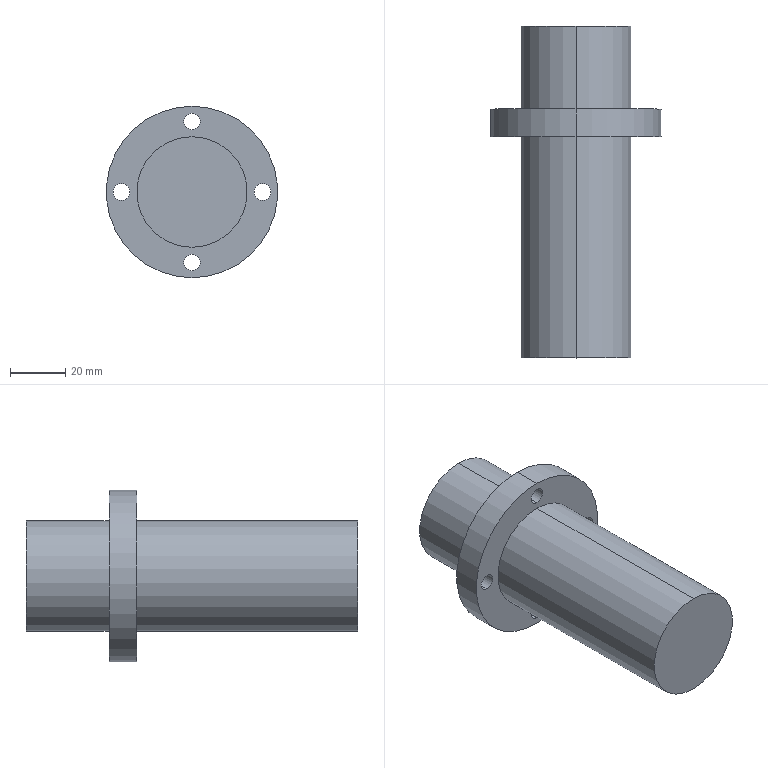Part | STEP file | slide bush dia25 | 1 solid | 21 faces | box 62 x 120 x 62 mm | volume 123111 mm3 | cylinder 16 | plane 5 | commonest cylinder face diameters 6 x8 40 x4 25 x2 62 x2
STEP:
#1=CARTESIAN_POINT('',(0.,0.,0.));
#2=DIRECTION('',(0.,0.,1.));
#3=DIRECTION('',(1.,0.,0.));
#4=AXIS2_PLACEMENT_3D('',#1,#2,#3);
#5=CARTESIAN_POINT('',(0.,80.,-22.5));
#6=VERTEX_POINT('',#5);
#7=CARTESIAN_POINT('',(0.,90.,-22.5));
#8=VERTEX_POINT('',#7);
#9=CARTESIAN_POINT('',(0.,90.,-22.5));
#10=DIRECTION('',(0.,1.,0.));
#11=VECTOR('',#10,1.);
#12=LINE('',#9,#11);
#13=CARTESIAN_POINT('',(0.,90.,-25.5));
#14=DIRECTION('',(0.,1.,0.));
#15=DIRECTION('',(0.,0.,1.));
#16=AXIS2_PLACEMENT_3D('',#13,#14,#15);
#17=CYLINDRICAL_SURFACE('',#16,3.);
#18=CARTESIAN_POINT('',(6.283,0.));
#19=DIRECTION('',(0.,1.));
#20=VECTOR('',#19,1.);
#21=LINE('',#18,#20);
#22=(GEOMETRIC_REPRESENTATION_CONTEXT(2)PARAMETRIC_REPRESENTATION_CONTEXT()REPRESENTATION_CONTEXT('',''));
#23=DEFINITIONAL_REPRESENTATION('',(#21),#22);
#24=PCURVE('',#17,#23);
#25=CARTESIAN_POINT('',(0.,90.,-25.5));
#26=DIRECTION('',(0.,1.,0.));
#27=DIRECTION('',(0.,0.,1.));
#28=AXIS2_PLACEMENT_3D('',#25,#26,#27);
#29=CYLINDRICAL_SURFACE('',#28,3.);
#30=CARTESIAN_POINT('',(0.,0.));
#31=DIRECTION('',(0.,1.));
#32=VECTOR('',#31,1.);
#33=LINE('',#30,#32);
#34=(GEOMETRIC_REPRESENTATION_CONTEXT(2)PARAMETRIC_REPRESENTATION_CONTEXT()REPRESENTATION_CONTEXT('',''));
#35=DEFINITIONAL_REPRESENTATION('',(#33),#34);
#36=PCURVE('',#29,#35);
#37=SURFACE_CURVE('',#12,(#24,#36),.PCURVE_S1.);
#38=EDGE_CURVE('',#6,#8,#37,.T.);
#39=ORIENTED_EDGE('',*,*,#38,.T.);
#40=CARTESIAN_POINT('',(0.,90.,-28.5));
#41=VERTEX_POINT('',#40);
#42=CARTESIAN_POINT('',(0.,90.,-25.5));
#43=DIRECTION('',(0.,1.,0.));
#44=DIRECTION('',(0.,0.,1.));
#45=AXIS2_PLACEMENT_3D('',#42,#43,#44);
#46=CIRCLE('',#45,3.);
#47=CARTESIAN_POINT('',(0.,0.));
#48=DIRECTION('',(1.,0.));
#49=VECTOR('',#48,1.);
#50=LINE('',#47,#49);
#51=(GEOMETRIC_REPRESENTATION_CONTEXT(2)PARAMETRIC_REPRESENTATION_CONTEXT()REPRESENTATION_CONTEXT('',''));
#52=DEFINITIONAL_REPRESENTATION('',(#50),#51);
#53=PCURVE('',#17,#52);
#54=CARTESIAN_POINT('',(0.,90.,0.));
#55=DIRECTION('',(0.,1.,0.));
#56=DIRECTION('',(0.,0.,1.));
#57=AXIS2_PLACEMENT_3D('',#54,#55,#56);
#58=PLANE('',#57);
#59=CARTESIAN_POINT('',(-25.5,0.));
#60=DIRECTION('',(1.,0.));
#61=AXIS2_PLACEMENT_2D('',#59,#60);
#62=CIRCLE('',#61,3.);
#63=(GEOMETRIC_REPRESENTATION_CONTEXT(2)PARAMETRIC_REPRESENTATION_CONTEXT()REPRESENTATION_CONTEXT('',''));
#64=DEFINITIONAL_REPRESENTATION('',(#62),#63);
#65=PCURVE('',#58,#64);
#66=SURFACE_CURVE('',#46,(#53,#65),.PCURVE_S1.);
#67=EDGE_CURVE('',#41,#8,#66,.T.);
#68=ORIENTED_EDGE('',*,*,#67,.F.);
#69=CARTESIAN_POINT('',(0.,80.,-28.5));
#70=VERTEX_POINT('',#69);
#71=CARTESIAN_POINT('',(0.,90.,-28.5));
#72=DIRECTION('',(0.,1.,0.));
#73=VECTOR('',#72,1.);
#74=LINE('',#71,#73);
#75=CARTESIAN_POINT('',(3.142,0.));
#76=DIRECTION('',(0.,1.));
#77=VECTOR('',#76,1.);
#78=LINE('',#75,#77);
#79=(GEOMETRIC_REPRESENTATION_CONTEXT(2)PARAMETRIC_REPRESENTATION_CONTEXT()REPRESENTATION_CONTEXT('',''));
#80=DEFINITIONAL_REPRESENTATION('',(#78),#79);
#81=PCURVE('',#17,#80);
#82=CARTESIAN_POINT('',(3.142,0.));
#83=DIRECTION('',(0.,1.));
#84=VECTOR('',#83,1.);
#85=LINE('',#82,#84);
#86=(GEOMETRIC_REPRESENTATION_CONTEXT(2)PARAMETRIC_REPRESENTATION_CONTEXT()REPRESENTATION_CONTEXT('',''));
#87=DEFINITIONAL_REPRESENTATION('',(#85),#86);
#88=PCURVE('',#29,#87);
#89=SURFACE_CURVE('',#74,(#81,#88),.PCURVE_S1.);
#90=EDGE_CURVE('',#70,#41,#89,.T.);
#91=ORIENTED_EDGE('',*,*,#90,.F.);
#92=CARTESIAN_POINT('',(0.,80.,-25.5));
#93=DIRECTION('',(0.,1.,0.));
#94=DIRECTION('',(0.,0.,1.));
#95=AXIS2_PLACEMENT_3D('',#92,#93,#94);
#96=CIRCLE('',#95,3.);
#97=CARTESIAN_POINT('',(0.,-10.));
#98=DIRECTION('',(1.,0.));
#99=VECTOR('',#98,1.);
#100=LINE('',#97,#99);
#101=(GEOMETRIC_REPRESENTATION_CONTEXT(2)PARAMETRIC_REPRESENTATION_CONTEXT()REPRESENTATION_CONTEXT('',''));
#102=DEFINITIONAL_REPRESENTATION('',(#100),#101);
#103=PCURVE('',#17,#102);
#104=CARTESIAN_POINT('',(0.,80.,0.));
#105=DIRECTION('',(0.,1.,0.));
#106=DIRECTION('',(0.,0.,1.));
#107=AXIS2_PLACEMENT_3D('',#104,#105,#106);
#108=PLANE('',#107);
#109=CARTESIAN_POINT('',(-25.5,0.));
#110=DIRECTION('',(1.,0.));
#111=AXIS2_PLACEMENT_2D('',#109,#110);
#112=CIRCLE('',#111,3.);
#113=(GEOMETRIC_REPRESENTATION_CONTEXT(2)PARAMETRIC_REPRESENTATION_CONTEXT()REPRESENTATION_CONTEXT('',''));
#114=DEFINITIONAL_REPRESENTATION('',(#112),#113);
#115=PCURVE('',#108,#114);
#116=SURFACE_CURVE('',#96,(#103,#115),.PCURVE_S1.);
#117=EDGE_CURVE('',#70,#6,#116,.T.);
#118=ORIENTED_EDGE('',*,*,#117,.T.);
#119=EDGE_LOOP('',(#39,#68,#91,#118));
#120=FACE_BOUND('',#119,.F.);
#121=ADVANCED_FACE('',(#120),#17,.F.);
#122=CARTESIAN_POINT('',(0.,80.,28.5));
#123=VERTEX_POINT('',#122);
#124=CARTESIAN_POINT('',(0.,90.,28.5));
#125=VERTEX_POINT('',#124);
#126=CARTESIAN_POINT('',(0.,90.,28.5));
#127=DIRECTION('',(0.,1.,0.));
#128=VECTOR('',#127,1.);
#129=LINE('',#126,#128);
#130=CARTESIAN_POINT('',(0.,90.,25.5));
#131=DIRECTION('',(0.,1.,0.));
#132=DIRECTION('',(0.,0.,1.));
#133=AXIS2_PLACEMENT_3D('',#130,#131,#132);
#134=CYLINDRICAL_SURFACE('',#133,3.);
#135=CARTESIAN_POINT('',(6.283,0.));
#136=DIRECTION('',(0.,1.));
#137=VECTOR('',#136,1.);
#138=LINE('',#135,#137);
#139=(GEOMETRIC_REPRESENTATION_CONTEXT(2)PARAMETRIC_REPRESENTATION_CONTEXT()REPRESENTATION_CONTEXT('',''));
#140=DEFINITIONAL_REPRESENTATION('',(#138),#139);
#141=PCURVE('',#134,#140);
#142=CARTESIAN_POINT('',(0.,90.,25.5));
#143=DIRECTION('',(0.,1.,0.));
#144=DIRECTION('',(0.,0.,1.));
#145=AXIS2_PLACEMENT_3D('',#142,#143,#144);
#146=CYLINDRICAL_SURFACE('',#145,3.);
#147=CARTESIAN_POINT('',(0.,0.));
#148=DIRECTION('',(0.,1.));
#149=VECTOR('',#148,1.);
#150=LINE('',#147,#149);
#151=(GEOMETRIC_REPRESENTATION_CONTEXT(2)PARAMETRIC_REPRESENTATION_CONTEXT()REPRESENTATION_CONTEXT('',''));
#152=DEFINITIONAL_REPRESENTATION('',(#150),#151);
#153=PCURVE('',#146,#152);
#154=SURFACE_CURVE('',#129,(#141,#153),.PCURVE_S1.);
#155=EDGE_CURVE('',#123,#125,#154,.T.);
#156=ORIENTED_EDGE('',*,*,#155,.T.);
#157=CARTESIAN_POINT('',(0.,90.,22.5));
#158=VERTEX_POINT('',#157);
#159=CARTESIAN_POINT('',(0.,90.,25.5));
#160=DIRECTION('',(0.,1.,0.));
#161=DIRECTION('',(0.,0.,1.));
#162=AXIS2_PLACEMENT_3D('',#159,#160,#161);
#163=CIRCLE('',#162,3.);
#164=CARTESIAN_POINT('',(0.,0.));
#165=DIRECTION('',(1.,0.));
#166=VECTOR('',#165,1.);
#167=LINE('',#164,#166);
#168=(GEOMETRIC_REPRESENTATION_CONTEXT(2)PARAMETRIC_REPRESENTATION_CONTEXT()REPRESENTATION_CONTEXT('',''));
#169=DEFINITIONAL_REPRESENTATION('',(#167),#168);
#170=PCURVE('',#134,#169);
#171=CARTESIAN_POINT('',(25.5,0.));
#172=DIRECTION('',(1.,0.));
#173=AXIS2_PLACEMENT_2D('',#171,#172);
#174=CIRCLE('',#173,3.);
#175=(GEOMETRIC_REPRESENTATION_CONTEXT(2)PARAMETRIC_REPRESENTATION_CONTEXT()REPRESENTATION_CONTEXT('',''));
#176=DEFINITIONAL_REPRESENTATION('',(#174),#175);
#177=PCURVE('',#58,#176);
#178=SURFACE_CURVE('',#163,(#170,#177),.PCURVE_S1.);
#179=EDGE_CURVE('',#158,#125,#178,.T.);
#180=ORIENTED_EDGE('',*,*,#179,.F.);
#181=CARTESIAN_POINT('',(0.,80.,22.5));
#182=VERTEX_POINT('',#181);
#183=CARTESIAN_POINT('',(0.,90.,22.5));
#184=DIRECTION('',(0.,1.,0.));
#185=VECTOR('',#184,1.);
#186=LINE('',#183,#185);
#187=CARTESIAN_POINT('',(3.142,0.));
#188=DIRECTION('',(0.,1.));
#189=VECTOR('',#188,1.);
#190=LINE('',#187,#189);
#191=(GEOMETRIC_REPRESENTATION_CONTEXT(2)PARAMETRIC_REPRESENTATION_CONTEXT()REPRESENTATION_CONTEXT('',''));
#192=DEFINITIONAL_REPRESENTATION('',(#190),#191);
#193=PCURVE('',#134,#192);
#194=CARTESIAN_POINT('',(3.142,0.));
#195=DIRECTION('',(0.,1.));
#196=VECTOR('',#195,1.);
#197=LINE('',#194,#196);
#198=(GEOMETRIC_REPRESENTATION_CONTEXT(2)PARAMETRIC_REPRESENTATION_CONTEXT()REPRESENTATION_CONTEXT('',''));
#199=DEFINITIONAL_REPRESENTATION('',(#197),#198);
#200=PCURVE('',#146,#199);
#201=SURFACE_CURVE('',#186,(#193,#200),.PCURVE_S1.);
#202=EDGE_CURVE('',#182,#158,#201,.T.);
#203=ORIENTED_EDGE('',*,*,#202,.F.);
#204=CARTESIAN_POINT('',(0.,80.,25.5));
#205=DIRECTION('',(0.,1.,0.));
#206=DIRECTION('',(0.,0.,1.));
#207=AXIS2_PLACEMENT_3D('',#204,#205,#206);
#208=CIRCLE('',#207,3.);
#209=CARTESIAN_POINT('',(0.,-10.));
#210=DIRECTION('',(1.,0.));
#211=VECTOR('',#210,1.);
#212=LINE('',#209,#211);
#213=(GEOMETRIC_REPRESENTATION_CONTEXT(2)PARAMETRIC_REPRESENTATION_CONTEXT()REPRESENTATION_CONTEXT('',''));
#214=DEFINITIONAL_REPRESENTATION('',(#212),#213);
#215=PCURVE('',#134,#214);
#216=CARTESIAN_POINT('',(25.5,0.));
#217=DIRECTION('',(1.,0.));
#218=AXIS2_PLACEMENT_2D('',#216,#217);
#219=CIRCLE('',#218,3.);
#220=(GEOMETRIC_REPRESENTATION_CONTEXT(2)PARAMETRIC_REPRESENTATION_CONTEXT()REPRESENTATION_CONTEXT('',''));
#221=DEFINITIONAL_REPRESENTATION('',(#219),#220);
#222=PCURVE('',#108,#221);
#223=SURFACE_CURVE('',#208,(#215,#222),.PCURVE_S1.);
#224=EDGE_CURVE('',#182,#123,#223,.T.);
#225=ORIENTED_EDGE('',*,*,#224,.T.);
#226=EDGE_LOOP('',(#156,#180,#203,#225));
#227=FACE_BOUND('',#226,.F.);
#228=ADVANCED_FACE('',(#227),#134,.F.);
#229=CARTESIAN_POINT('',(-25.5,80.,3.));
#230=VERTEX_POINT('',#229);
#231=CARTESIAN_POINT('',(-25.5,90.,3.));
#232=VERTEX_POINT('',#231);
#233=CARTESIAN_POINT('',(-25.5,90.,3.));
#234=DIRECTION('',(0.,1.,0.));
#235=VECTOR('',#234,1.);
#236=LINE('',#233,#235);
#237=CARTESIAN_POINT('',(-25.5,90.,0.));
#238=DIRECTION('',(0.,1.,0.));
#239=DIRECTION('',(0.,0.,1.));
#240=AXIS2_PLACEMENT_3D('',#237,#238,#239);
#241=CYLINDRICAL_SURFACE('',#240,3.);
#242=CARTESIAN_POINT('',(6.283,0.));
#243=DIRECTION('',(0.,1.));
#244=VECTOR('',#243,1.);
#245=LINE('',#242,#244);
#246=(GEOMETRIC_REPRESENTATION_CONTEXT(2)PARAMETRIC_REPRESENTATION_CONTEXT()REPRESENTATION_CONTEXT('',''));
#247=DEFINITIONAL_REPRESENTATION('',(#245),#246);
#248=PCURVE('',#241,#247);
#249=CARTESIAN_POINT('',(-25.5,90.,0.));
#250=DIRECTION('',(0.,1.,0.));
#251=DIRECTION('',(0.,0.,1.));
#252=AXIS2_PLACEMENT_3D('',#249,#250,#251);
#253=CYLINDRICAL_SURFACE('',#252,3.);
#254=CARTESIAN_POINT('',(0.,0.));
#255=DIRECTION('',(0.,1.));
#256=VECTOR('',#255,1.);
#257=LINE('',#254,#256);
#258=(GEOMETRIC_REPRESENTATION_CONTEXT(2)PARAMETRIC_REPRESENTATION_CONTEXT()REPRESENTATION_CONTEXT('',''));
#259=DEFINITIONAL_REPRESENTATION('',(#257),#258);
#260=PCURVE('',#253,#259);
#261=SURFACE_CURVE('',#236,(#248,#260),.PCURVE_S1.);
#262=EDGE_CURVE('',#230,#232,#261,.T.);
#263=ORIENTED_EDGE('',*,*,#262,.T.);
#264=CARTESIAN_POINT('',(-25.5,90.,-3.));
#265=VERTEX_POINT('',#264);
#266=CARTESIAN_POINT('',(-25.5,90.,0.));
#267=DIRECTION('',(0.,1.,0.));
#268=DIRECTION('',(0.,0.,1.));
#269=AXIS2_PLACEMENT_3D('',#266,#267,#268);
#270=CIRCLE('',#269,3.);
#271=CARTESIAN_POINT('',(0.,0.));
#272=DIRECTION('',(1.,0.));
#273=VECTOR('',#272,1.);
#274=LINE('',#271,#273);
#275=(GEOMETRIC_REPRESENTATION_CONTEXT(2)PARAMETRIC_REPRESENTATION_CONTEXT()REPRESENTATION_CONTEXT('',''));
#276=DEFINITIONAL_REPRESENTATION('',(#274),#275);
#277=PCURVE('',#241,#276);
#278=CARTESIAN_POINT('',(0.,-25.5));
#279=DIRECTION('',(1.,0.));
#280=AXIS2_PLACEMENT_2D('',#278,#279);
#281=CIRCLE('',#280,3.);
#282=(GEOMETRIC_REPRESENTATION_CONTEXT(2)PARAMETRIC_REPRESENTATION_CONTEXT()REPRESENTATION_CONTEXT('',''));
#283=DEFINITIONAL_REPRESENTATION('',(#281),#282);
#284=PCURVE('',#58,#283);
#285=SURFACE_CURVE('',#270,(#277,#284),.PCURVE_S1.);
#286=EDGE_CURVE('',#265,#232,#285,.T.);
#287=ORIENTED_EDGE('',*,*,#286,.F.);
#288=CARTESIAN_POINT('',(-25.5,80.,-3.));
#289=VERTEX_POINT('',#288);
#290=CARTESIAN_POINT('',(-25.5,90.,-3.));
#291=DIRECTION('',(0.,1.,0.));
#292=VECTOR('',#291,1.);
#293=LINE('',#290,#292);
#294=CARTESIAN_POINT('',(3.142,0.));
#295=DIRECTION('',(0.,1.));
#296=VECTOR('',#295,1.);
#297=LINE('',#294,#296);
#298=(GEOMETRIC_REPRESENTATION_CONTEXT(2)PARAMETRIC_REPRESENTATION_CONTEXT()REPRESENTATION_CONTEXT('',''));
#299=DEFINITIONAL_REPRESENTATION('',(#297),#298);
#300=PCURVE('',#241,#299);
#301=CARTESIAN_POINT('',(3.142,0.));
#302=DIRECTION('',(0.,1.));
#303=VECTOR('',#302,1.);
#304=LINE('',#301,#303);
#305=(GEOMETRIC_REPRESENTATION_CONTEXT(2)PARAMETRIC_REPRESENTATION_CONTEXT()REPRESENTATION_CONTEXT('',''));
#306=DEFINITIONAL_REPRESENTATION('',(#304),#305);
#307=PCURVE('',#253,#306);
#308=SURFACE_CURVE('',#293,(#300,#307),.PCURVE_S1.);
#309=EDGE_CURVE('',#289,#265,#308,.T.);
#310=ORIENTED_EDGE('',*,*,#309,.F.);
#311=CARTESIAN_POINT('',(-25.5,80.,0.));
#312=DIRECTION('',(0.,1.,0.));
#313=DIRECTION('',(0.,0.,1.));
#314=AXIS2_PLACEMENT_3D('',#311,#312,#313);
#315=CIRCLE('',#314,3.);
#316=CARTESIAN_POINT('',(0.,-10.));
#317=DIRECTION('',(1.,0.));
#318=VECTOR('',#317,1.);
#319=LINE('',#316,#318);
#320=(GEOMETRIC_REPRESENTATION_CONTEXT(2)PARAMETRIC_REPRESENTATION_CONTEXT()REPRESENTATION_CONTEXT('',''));
#321=DEFINITIONAL_REPRESENTATION('',(#319),#320);
#322=PCURVE('',#241,#321);
#323=CARTESIAN_POINT('',(0.,-25.5));
#324=DIRECTION('',(1.,0.));
#325=AXIS2_PLACEMENT_2D('',#323,#324);
#326=CIRCLE('',#325,3.);
#327=(GEOMETRIC_REPRESENTATION_CONTEXT(2)PARAMETRIC_REPRESENTATION_CONTEXT()REPRESENTATION_CONTEXT('',''));
#328=DEFINITIONAL_REPRESENTATION('',(#326),#327);
#329=PCURVE('',#108,#328);
#330=SURFACE_CURVE('',#315,(#322,#329),.PCURVE_S1.);
#331=EDGE_CURVE('',#289,#230,#330,.T.);
#332=ORIENTED_EDGE('',*,*,#331,.T.);
#333=EDGE_LOOP('',(#263,#287,#310,#332));
#334=FACE_BOUND('',#333,.F.);
#335=ADVANCED_FACE('',(#334),#241,.F.);
#336=CARTESIAN_POINT('',(25.5,80.,3.));
#337=VERTEX_POINT('',#336);
#338=CARTESIAN_POINT('',(25.5,90.,3.));
#339=VERTEX_POINT('',#338);
#340=CARTESIAN_POINT('',(25.5,90.,3.));
#341=DIRECTION('',(0.,1.,0.));
#342=VECTOR('',#341,1.);
#343=LINE('',#340,#342);
#344=CARTESIAN_POINT('',(25.5,90.,0.));
#345=DIRECTION('',(0.,1.,0.));
#346=DIRECTION('',(0.,0.,1.));
#347=AXIS2_PLACEMENT_3D('',#344,#345,#346);
#348=CYLINDRICAL_SURFACE('',#347,3.);
#349=CARTESIAN_POINT('',(6.283,0.));
#350=DIRECTION('',(0.,1.));
#351=VECTOR('',#350,1.);
#352=LINE('',#349,#351);
#353=(GEOMETRIC_REPRESENTATION_CONTEXT(2)PARAMETRIC_REPRESENTATION_CONTEXT()REPRESENTATION_CONTEXT('',''));
#354=DEFINITIONAL_REPRESENTATION('',(#352),#353);
#355=PCURVE('',#348,#354);
#356=CARTESIAN_POINT('',(25.5,90.,0.));
#357=DIRECTION('',(0.,1.,0.));
#358=DIRECTION('',(0.,0.,1.));
#359=AXIS2_PLACEMENT_3D('',#356,#357,#358);
#360=CYLINDRICAL_SURFACE('',#359,3.);
#361=CARTESIAN_POINT('',(0.,0.));
#362=DIRECTION('',(0.,1.));
#363=VECTOR('',#362,1.);
#364=LINE('',#361,#363);
#365=(GEOMETRIC_REPRESENTATION_CONTEXT(2)PARAMETRIC_REPRESENTATION_CONTEXT()REPRESENTATION_CONTEXT('',''));
#366=DEFINITIONAL_REPRESENTATION('',(#364),#365);
#367=PCURVE('',#360,#366);
#368=SURFACE_CURVE('',#343,(#355,#367),.PCURVE_S1.);
#369=EDGE_CURVE('',#337,#339,#368,.T.);
#370=ORIENTED_EDGE('',*,*,#369,.T.);
#371=CARTESIAN_POINT('',(25.5,90.,-3.));
#372=VERTEX_POINT('',#371);
#373=CARTESIAN_POINT('',(25.5,90.,0.));
#374=DIRECTION('',(0.,1.,0.));
#375=DIRECTION('',(0.,0.,1.));
#376=AXIS2_PLACEMENT_3D('',#373,#374,#375);
#377=CIRCLE('',#376,3.);
#378=CARTESIAN_POINT('',(0.,0.));
#379=DIRECTION('',(1.,0.));
#380=VECTOR('',#379,1.);
#381=LINE('',#378,#380);
#382=(GEOMETRIC_REPRESENTATION_CONTEXT(2)PARAMETRIC_REPRESENTATION_CONTEXT()REPRESENTATION_CONTEXT('',''));
#383=DEFINITIONAL_REPRESENTATION('',(#381),#382);
#384=PCURVE('',#348,#383);
#385=CARTESIAN_POINT('',(0.,25.5));
#386=DIRECTION('',(1.,0.));
#387=AXIS2_PLACEMENT_2D('',#385,#386);
#388=CIRCLE('',#387,3.);
#389=(GEOMETRIC_REPRESENTATION_CONTEXT(2)PARAMETRIC_REPRESENTATION_CONTEXT()REPRESENTATION_CONTEXT('',''));
#390=DEFINITIONAL_REPRESENTATION('',(#388),#389);
#391=PCURVE('',#58,#390);
#392=SURFACE_CURVE('',#377,(#384,#391),.PCURVE_S1.);
#393=EDGE_CURVE('',#372,#339,#392,.T.);
#394=ORIENTED_EDGE('',*,*,#393,.F.);
#395=CARTESIAN_POINT('',(25.5,80.,-3.));
#396=VERTEX_POINT('',#395);
#397=CARTESIAN_POINT('',(25.5,90.,-3.));
#398=DIRECTION('',(0.,1.,0.));
#399=VECTOR('',#398,1.);
#400=LINE('',#397,#399);
#401=CARTESIAN_POINT('',(3.142,0.));
#402=DIRECTION('',(0.,1.));
#403=VECTOR('',#402,1.);
#404=LINE('',#401,#403);
#405=(GEOMETRIC_REPRESENTATION_CONTEXT(2)PARAMETRIC_REPRESENTATION_CONTEXT()REPRESENTATION_CONTEXT('',''));
#406=DEFINITIONAL_REPRESENTATION('',(#404),#405);
#407=PCURVE('',#348,#406);
#408=CARTESIAN_POINT('',(3.142,0.));
#409=DIRECTION('',(0.,1.));
#410=VECTOR('',#409,1.);
#411=LINE('',#408,#410);
#412=(GEOMETRIC_REPRESENTATION_CONTEXT(2)PARAMETRIC_REPRESENTATION_CONTEXT()REPRESENTATION_CONTEXT('',''));
#413=DEFINITIONAL_REPRESENTATION('',(#411),#412);
#414=PCURVE('',#360,#413);
#415=SURFACE_CURVE('',#400,(#407,#414),.PCURVE_S1.);
#416=EDGE_CURVE('',#396,#372,#415,.T.);
#417=ORIENTED_EDGE('',*,*,#416,.F.);
#418=CARTESIAN_POINT('',(25.5,80.,0.));
#419=DIRECTION('',(0.,1.,0.));
#420=DIRECTION('',(0.,0.,1.));
#421=AXIS2_PLACEMENT_3D('',#418,#419,#420);
#422=CIRCLE('',#421,3.);
#423=CARTESIAN_POINT('',(0.,-10.));
#424=DIRECTION('',(1.,0.));
#425=VECTOR('',#424,1.);
#426=LINE('',#423,#425);
#427=(GEOMETRIC_REPRESENTATION_CONTEXT(2)PARAMETRIC_REPRESENTATION_CONTEXT()REPRESENTATION_CONTEXT('',''));
#428=DEFINITIONAL_REPRESENTATION('',(#426),#427);
#429=PCURVE('',#348,#428);
#430=CARTESIAN_POINT('',(0.,25.5));
#431=DIRECTION('',(1.,0.));
#432=AXIS2_PLACEMENT_2D('',#430,#431);
#433=CIRCLE('',#432,3.);
#434=(GEOMETRIC_REPRESENTATION_CONTEXT(2)PARAMETRIC_REPRESENTATION_CONTEXT()REPRESENTATION_CONTEXT('',''));
#435=DEFINITIONAL_REPRESENTATION('',(#433),#434);
#436=PCURVE('',#108,#435);
#437=SURFACE_CURVE('',#422,(#429,#436),.PCURVE_S1.);
#438=EDGE_CURVE('',#396,#337,#437,.T.);
#439=ORIENTED_EDGE('',*,*,#438,.T.);
#440=EDGE_LOOP('',(#370,#394,#417,#439));
#441=FACE_BOUND('',#440,.F.);
#442=ADVANCED_FACE('',(#441),#348,.F.);
#443=CARTESIAN_POINT('',(0.,30.,12.5));
#444=VERTEX_POINT('',#443);
#445=CARTESIAN_POINT('',(0.,120.,12.5));
#446=VERTEX_POINT('',#445);
#447=CARTESIAN_POINT('',(0.,30.,12.5));
#448=DIRECTION('',(0.,1.,0.));
#449=VECTOR('',#448,1.);
#450=LINE('',#447,#449);
#451=CARTESIAN_POINT('',(0.,30.,0.));
#452=DIRECTION('',(0.,1.,0.));
#453=DIRECTION('',(0.,0.,1.));
#454=AXIS2_PLACEMENT_3D('',#451,#452,#453);
#455=CYLINDRICAL_SURFACE('',#454,12.5);
#456=CARTESIAN_POINT('',(6.283,0.));
#457=DIRECTION('',(0.,1.));
#458=VECTOR('',#457,1.);
#459=LINE('',#456,#458);
#460=(GEOMETRIC_REPRESENTATION_CONTEXT(2)PARAMETRIC_REPRESENTATION_CONTEXT()REPRESENTATION_CONTEXT('',''));
#461=DEFINITIONAL_REPRESENTATION('',(#459),#460);
#462=PCURVE('',#455,#461);
#463=CARTESIAN_POINT('',(0.,30.,0.));
#464=DIRECTION('',(0.,1.,0.));
#465=DIRECTION('',(0.,0.,1.));
#466=AXIS2_PLACEMENT_3D('',#463,#464,#465);
#467=CYLINDRICAL_SURFACE('',#466,12.5);
#468=CARTESIAN_POINT('',(0.,0.));
#469=DIRECTION('',(0.,1.));
#470=VECTOR('',#469,1.);
#471=LINE('',#468,#470);
#472=(GEOMETRIC_REPRESENTATION_CONTEXT(2)PARAMETRIC_REPRESENTATION_CONTEXT()REPRESENTATION_CONTEXT('',''));
#473=DEFINITIONAL_REPRESENTATION('',(#471),#472);
#474=PCURVE('',#467,#473);
#475=SURFACE_CURVE('',#450,(#462,#474),.PCURVE_S1.);
#476=EDGE_CURVE('',#444,#446,#475,.T.);
#477=ORIENTED_EDGE('',*,*,#476,.T.);
#478=CARTESIAN_POINT('',(0.,120.,-12.5));
#479=VERTEX_POINT('',#478);
#480=CARTESIAN_POINT('',(0.,120.,0.));
#481=DIRECTION('',(0.,1.,0.));
#482=DIRECTION('',(0.,0.,1.));
#483=AXIS2_PLACEMENT_3D('',#480,#481,#482);
#484=CIRCLE('',#483,12.5);
#485=CARTESIAN_POINT('',(0.,90.));
#486=DIRECTION('',(1.,0.));
#487=VECTOR('',#486,1.);
#488=LINE('',#485,#487);
#489=(GEOMETRIC_REPRESENTATION_CONTEXT(2)PARAMETRIC_REPRESENTATION_CONTEXT()REPRESENTATION_CONTEXT('',''));
#490=DEFINITIONAL_REPRESENTATION('',(#488),#489);
#491=PCURVE('',#455,#490);
#492=CARTESIAN_POINT('',(0.,120.,0.));
#493=DIRECTION('',(0.,1.,0.));
#494=DIRECTION('',(0.,0.,1.));
#495=AXIS2_PLACEMENT_3D('',#492,#493,#494);
#496=PLANE('',#495);
#497=CARTESIAN_POINT('',(0.,0.));
#498=DIRECTION('',(1.,0.));
#499=AXIS2_PLACEMENT_2D('',#497,#498);
#500=CIRCLE('',#499,12.5);
#501=(GEOMETRIC_REPRESENTATION_CONTEXT(2)PARAMETRIC_REPRESENTATION_CONTEXT()REPRESENTATION_CONTEXT('',''));
#502=DEFINITIONAL_REPRESENTATION('',(#500),#501);
#503=PCURVE('',#496,#502);
#504=SURFACE_CURVE('',#484,(#491,#503),.PCURVE_S1.);
#505=EDGE_CURVE('',#479,#446,#504,.T.);
#506=ORIENTED_EDGE('',*,*,#505,.F.);
#507=CARTESIAN_POINT('',(0.,30.,-12.5));
#508=VERTEX_POINT('',#507);
#509=CARTESIAN_POINT('',(0.,30.,-12.5));
#510=DIRECTION('',(0.,1.,0.));
#511=VECTOR('',#510,1.);
#512=LINE('',#509,#511);
#513=CARTESIAN_POINT('',(3.142,0.));
#514=DIRECTION('',(0.,1.));
#515=VECTOR('',#514,1.);
#516=LINE('',#513,#515);
#517=(GEOMETRIC_REPRESENTATION_CONTEXT(2)PARAMETRIC_REPRESENTATION_CONTEXT()REPRESENTATION_CONTEXT('',''));
#518=DEFINITIONAL_REPRESENTATION('',(#516),#517);
#519=PCURVE('',#455,#518);
#520=CARTESIAN_POINT('',(3.142,0.));
#521=DIRECTION('',(0.,1.));
#522=VECTOR('',#521,1.);
#523=LINE('',#520,#522);
#524=(GEOMETRIC_REPRESENTATION_CONTEXT(2)PARAMETRIC_REPRESENTATION_CONTEXT()REPRESENTATION_CONTEXT('',''));
#525=DEFINITIONAL_REPRESENTATION('',(#523),#524);
#526=PCURVE('',#467,#525);
#527=SURFACE_CURVE('',#512,(#519,#526),.PCURVE_S1.);
#528=EDGE_CURVE('',#508,#479,#527,.T.);
#529=ORIENTED_EDGE('',*,*,#528,.F.);
#530=CARTESIAN_POINT('',(0.,30.,0.));
#531=DIRECTION('',(0.,1.,0.));
#532=DIRECTION('',(0.,0.,1.));
#533=AXIS2_PLACEMENT_3D('',#530,#531,#532);
#534=CIRCLE('',#533,12.5);
#535=CARTESIAN_POINT('',(0.,0.));
#536=DIRECTION('',(1.,0.));
#537=VECTOR('',#536,1.);
#538=LINE('',#535,#537);
#539=(GEOMETRIC_REPRESENTATION_CONTEXT(2)PARAMETRIC_REPRESENTATION_CONTEXT()REPRESENTATION_CONTEXT('',''));
#540=DEFINITIONAL_REPRESENTATION('',(#538),#539);
#541=PCURVE('',#455,#540);
#542=CARTESIAN_POINT('',(0.,30.,0.));
#543=DIRECTION('',(0.,1.,0.));
#544=DIRECTION('',(0.,0.,1.));
#545=AXIS2_PLACEMENT_3D('',#542,#543,#544);
#546=PLANE('',#545);
#547=CARTESIAN_POINT('',(0.,0.));
#548=DIRECTION('',(1.,0.));
#549=AXIS2_PLACEMENT_2D('',#547,#548);
#550=CIRCLE('',#549,12.5);
#551=(GEOMETRIC_REPRESENTATION_CONTEXT(2)PARAMETRIC_REPRESENTATION_CONTEXT()REPRESENTATION_CONTEXT('',''));
#552=DEFINITIONAL_REPRESENTATION('',(#550),#551);
#553=PCURVE('',#546,#552);
#554=SURFACE_CURVE('',#534,(#541,#553),.PCURVE_S1.);
#555=EDGE_CURVE('',#508,#444,#554,.T.);
#556=ORIENTED_EDGE('',*,*,#555,.T.);
#557=EDGE_LOOP('',(#477,#506,#529,#556));
#558=FACE_BOUND('',#557,.F.);
#559=ADVANCED_FACE('',(#558),#455,.F.);
#560=CARTESIAN_POINT('',(0.,120.,20.));
#561=VERTEX_POINT('',#560);
#562=CARTESIAN_POINT('',(0.,120.,-20.));
#563=VERTEX_POINT('',#562);
#564=CARTESIAN_POINT('',(0.,120.,0.));
#565=DIRECTION('',(0.,1.,0.));
#566=DIRECTION('',(0.,0.,1.));
#567=AXIS2_PLACEMENT_3D('',#564,#565,#566);
#568=CIRCLE('',#567,20.);
#569=CARTESIAN_POINT('',(0.,120.,0.));
#570=DIRECTION('',(0.,-1.,0.));
#571=DIRECTION('',(0.,0.,-1.));
#572=AXIS2_PLACEMENT_3D('',#569,#570,#571);
#573=CYLINDRICAL_SURFACE('',#572,20.);
#574=CARTESIAN_POINT('',(3.142,0.));
#575=DIRECTION('',(-1.,0.));
#576=VECTOR('',#575,1.);
#577=LINE('',#574,#576);
#578=(GEOMETRIC_REPRESENTATION_CONTEXT(2)PARAMETRIC_REPRESENTATION_CONTEXT()REPRESENTATION_CONTEXT('',''));
#579=DEFINITIONAL_REPRESENTATION('',(#577),#578);
#580=PCURVE('',#573,#579);
#581=CARTESIAN_POINT('',(0.,0.));
#582=DIRECTION('',(1.,0.));
#583=AXIS2_PLACEMENT_2D('',#581,#582);
#584=CIRCLE('',#583,20.);
#585=(GEOMETRIC_REPRESENTATION_CONTEXT(2)PARAMETRIC_REPRESENTATION_CONTEXT()REPRESENTATION_CONTEXT('',''));
#586=DEFINITIONAL_REPRESENTATION('',(#584),#585);
#587=PCURVE('',#496,#586);
#588=SURFACE_CURVE('',#568,(#580,#587),.PCURVE_S1.);
#589=EDGE_CURVE('',#561,#563,#588,.T.);
#590=ORIENTED_EDGE('',*,*,#589,.F.);
#591=CARTESIAN_POINT('',(0.,90.,20.));
#592=VERTEX_POINT('',#591);
#593=CARTESIAN_POINT('',(0.,120.,20.));
#594=DIRECTION('',(0.,-1.,0.));
#595=VECTOR('',#594,1.);
#596=LINE('',#593,#595);
#597=CARTESIAN_POINT('',(3.142,0.));
#598=DIRECTION('',(0.,1.));
#599=VECTOR('',#598,1.);
#600=LINE('',#597,#599);
#601=(GEOMETRIC_REPRESENTATION_CONTEXT(2)PARAMETRIC_REPRESENTATION_CONTEXT()REPRESENTATION_CONTEXT('',''));
#602=DEFINITIONAL_REPRESENTATION('',(#600),#601);
#603=PCURVE('',#573,#602);
#604=CARTESIAN_POINT('',(0.,120.,0.));
#605=DIRECTION('',(0.,-1.,0.));
#606=DIRECTION('',(0.,0.,-1.));
#607=AXIS2_PLACEMENT_3D('',#604,#605,#606);
#608=CYLINDRICAL_SURFACE('',#607,20.);
#609=CARTESIAN_POINT('',(3.142,0.));
#610=DIRECTION('',(0.,1.));
#611=VECTOR('',#610,1.);
#612=LINE('',#609,#611);
#613=(GEOMETRIC_REPRESENTATION_CONTEXT(2)PARAMETRIC_REPRESENTATION_CONTEXT()REPRESENTATION_CONTEXT('',''));
#614=DEFINITIONAL_REPRESENTATION('',(#612),#613);
#615=PCURVE('',#608,#614);
#616=SURFACE_CURVE('',#596,(#603,#615),.PCURVE_S1.);
#617=EDGE_CURVE('',#561,#592,#616,.T.);
#618=ORIENTED_EDGE('',*,*,#617,.T.);
#619=CARTESIAN_POINT('',(0.,90.,-20.));
#620=VERTEX_POINT('',#619);
#621=CARTESIAN_POINT('',(0.,90.,0.));
#622=DIRECTION('',(0.,1.,0.));
#623=DIRECTION('',(0.,0.,1.));
#624=AXIS2_PLACEMENT_3D('',#621,#622,#623);
#625=CIRCLE('',#624,20.);
#626=CARTESIAN_POINT('',(3.142,30.));
#627=DIRECTION('',(-1.,0.));
#628=VECTOR('',#627,1.);
#629=LINE('',#626,#628);
#630=(GEOMETRIC_REPRESENTATION_CONTEXT(2)PARAMETRIC_REPRESENTATION_CONTEXT()REPRESENTATION_CONTEXT('',''));
#631=DEFINITIONAL_REPRESENTATION('',(#629),#630);
#632=PCURVE('',#573,#631);
#633=CARTESIAN_POINT('',(0.,0.));
#634=DIRECTION('',(1.,0.));
#635=AXIS2_PLACEMENT_2D('',#633,#634);
#636=CIRCLE('',#635,20.);
#637=(GEOMETRIC_REPRESENTATION_CONTEXT(2)PARAMETRIC_REPRESENTATION_CONTEXT()REPRESENTATION_CONTEXT('',''));
#638=DEFINITIONAL_REPRESENTATION('',(#636),#637);
#639=PCURVE('',#58,#638);
#640=SURFACE_CURVE('',#625,(#632,#639),.PCURVE_S1.);
#641=EDGE_CURVE('',#592,#620,#640,.T.);
#642=ORIENTED_EDGE('',*,*,#641,.T.);
#643=CARTESIAN_POINT('',(0.,120.,-20.));
#644=DIRECTION('',(0.,-1.,0.));
#645=VECTOR('',#644,1.);
#646=LINE('',#643,#645);
#647=CARTESIAN_POINT('',(0.,0.));
#648=DIRECTION('',(0.,1.));
#649=VECTOR('',#648,1.);
#650=LINE('',#647,#649);
#651=(GEOMETRIC_REPRESENTATION_CONTEXT(2)PARAMETRIC_REPRESENTATION_CONTEXT()REPRESENTATION_CONTEXT('',''));
#652=DEFINITIONAL_REPRESENTATION('',(#650),#651);
#653=PCURVE('',#573,#652);
#654=CARTESIAN_POINT('',(6.283,0.));
#655=DIRECTION('',(0.,1.));
#656=VECTOR('',#655,1.);
#657=LINE('',#654,#656);
#658=(GEOMETRIC_REPRESENTATION_CONTEXT(2)PARAMETRIC_REPRESENTATION_CONTEXT()REPRESENTATION_CONTEXT('',''));
#659=DEFINITIONAL_REPRESENTATION('',(#657),#658);
#660=PCURVE('',#608,#659);
#661=SURFACE_CURVE('',#646,(#653,#660),.PCURVE_S1.);
#662=EDGE_CURVE('',#563,#620,#661,.T.);
#663=ORIENTED_EDGE('',*,*,#662,.F.);
#664=EDGE_LOOP('',(#590,#618,#642,#663));
#665=FACE_BOUND('',#664,.T.);
#666=ADVANCED_FACE('',(#665),#573,.T.);
#667=CARTESIAN_POINT('',(0.,90.,31.));
#668=VERTEX_POINT('',#667);
#669=CARTESIAN_POINT('',(0.,90.,-31.));
#670=VERTEX_POINT('',#669);
#671=CARTESIAN_POINT('',(0.,90.,0.));
#672=DIRECTION('',(0.,1.,0.));
#673=DIRECTION('',(0.,0.,1.));
#674=AXIS2_PLACEMENT_3D('',#671,#672,#673);
#675=CIRCLE('',#674,31.);
#676=CARTESIAN_POINT('',(0.,90.,0.));
#677=DIRECTION('',(0.,-1.,0.));
#678=DIRECTION('',(0.,0.,-1.));
#679=AXIS2_PLACEMENT_3D('',#676,#677,#678);
#680=CYLINDRICAL_SURFACE('',#679,31.);
#681=CARTESIAN_POINT('',(3.142,0.));
#682=DIRECTION('',(-1.,0.));
#683=VECTOR('',#682,1.);
#684=LINE('',#681,#683);
#685=(GEOMETRIC_REPRESENTATION_CONTEXT(2)PARAMETRIC_REPRESENTATION_CONTEXT()REPRESENTATION_CONTEXT('',''));
#686=DEFINITIONAL_REPRESENTATION('',(#684),#685);
#687=PCURVE('',#680,#686);
#688=CARTESIAN_POINT('',(0.,0.));
#689=DIRECTION('',(1.,0.));
#690=AXIS2_PLACEMENT_2D('',#688,#689);
#691=CIRCLE('',#690,31.);
#692=(GEOMETRIC_REPRESENTATION_CONTEXT(2)PARAMETRIC_REPRESENTATION_CONTEXT()REPRESENTATION_CONTEXT('',''));
#693=DEFINITIONAL_REPRESENTATION('',(#691),#692);
#694=PCURVE('',#58,#693);
#695=SURFACE_CURVE('',#675,(#687,#694),.PCURVE_S1.);
#696=EDGE_CURVE('',#668,#670,#695,.T.);
#697=ORIENTED_EDGE('',*,*,#696,.F.);
#698=CARTESIAN_POINT('',(0.,80.,31.));
#699=VERTEX_POINT('',#698);
#700=CARTESIAN_POINT('',(0.,90.,31.));
#701=DIRECTION('',(0.,-1.,0.));
#702=VECTOR('',#701,1.);
#703=LINE('',#700,#702);
#704=CARTESIAN_POINT('',(3.142,0.));
#705=DIRECTION('',(0.,1.));
#706=VECTOR('',#705,1.);
#707=LINE('',#704,#706);
#708=(GEOMETRIC_REPRESENTATION_CONTEXT(2)PARAMETRIC_REPRESENTATION_CONTEXT()REPRESENTATION_CONTEXT('',''));
#709=DEFINITIONAL_REPRESENTATION('',(#707),#708);
#710=PCURVE('',#680,#709);
#711=CARTESIAN_POINT('',(0.,90.,0.));
#712=DIRECTION('',(0.,-1.,0.));
#713=DIRECTION('',(0.,0.,-1.));
#714=AXIS2_PLACEMENT_3D('',#711,#712,#713);
#715=CYLINDRICAL_SURFACE('',#714,31.);
#716=CARTESIAN_POINT('',(3.142,0.));
#717=DIRECTION('',(0.,1.));
#718=VECTOR('',#717,1.);
#719=LINE('',#716,#718);
#720=(GEOMETRIC_REPRESENTATION_CONTEXT(2)PARAMETRIC_REPRESENTATION_CONTEXT()REPRESENTATION_CONTEXT('',''));
#721=DEFINITIONAL_REPRESENTATION('',(#719),#720);
#722=PCURVE('',#715,#721);
#723=SURFACE_CURVE('',#703,(#710,#722),.PCURVE_S1.);
#724=EDGE_CURVE('',#668,#699,#723,.T.);
#725=ORIENTED_EDGE('',*,*,#724,.T.);
#726=CARTESIAN_POINT('',(0.,80.,-31.));
#727=VERTEX_POINT('',#726);
#728=CARTESIAN_POINT('',(0.,80.,0.));
#729=DIRECTION('',(0.,1.,0.));
#730=DIRECTION('',(0.,0.,1.));
#731=AXIS2_PLACEMENT_3D('',#728,#729,#730);
#732=CIRCLE('',#731,31.);
#733=CARTESIAN_POINT('',(3.142,10.));
#734=DIRECTION('',(-1.,0.));
#735=VECTOR('',#734,1.);
#736=LINE('',#733,#735);
#737=(GEOMETRIC_REPRESENTATION_CONTEXT(2)PARAMETRIC_REPRESENTATION_CONTEXT()REPRESENTATION_CONTEXT('',''));
#738=DEFINITIONAL_REPRESENTATION('',(#736),#737);
#739=PCURVE('',#680,#738);
#740=CARTESIAN_POINT('',(0.,0.));
#741=DIRECTION('',(1.,0.));
#742=AXIS2_PLACEMENT_2D('',#740,#741);
#743=CIRCLE('',#742,31.);
#744=(GEOMETRIC_REPRESENTATION_CONTEXT(2)PARAMETRIC_REPRESENTATION_CONTEXT()REPRESENTATION_CONTEXT('',''));
#745=DEFINITIONAL_REPRESENTATION('',(#743),#744);
#746=PCURVE('',#108,#745);
#747=SURFACE_CURVE('',#732,(#739,#746),.PCURVE_S1.);
#748=EDGE_CURVE('',#699,#727,#747,.T.);
#749=ORIENTED_EDGE('',*,*,#748,.T.);
#750=CARTESIAN_POINT('',(0.,90.,-31.));
#751=DIRECTION('',(0.,-1.,0.));
#752=VECTOR('',#751,1.);
#753=LINE('',#750,#752);
#754=CARTESIAN_POINT('',(0.,0.));
#755=DIRECTION('',(0.,1.));
#756=VECTOR('',#755,1.);
#757=LINE('',#754,#756);
#758=(GEOMETRIC_REPRESENTATION_CONTEXT(2)PARAMETRIC_REPRESENTATION_CONTEXT()REPRESENTATION_CONTEXT('',''));
#759=DEFINITIONAL_REPRESENTATION('',(#757),#758);
#760=PCURVE('',#680,#759);
#761=CARTESIAN_POINT('',(6.283,0.));
#762=DIRECTION('',(0.,1.));
#763=VECTOR('',#762,1.);
#764=LINE('',#761,#763);
#765=(GEOMETRIC_REPRESENTATION_CONTEXT(2)PARAMETRIC_REPRESENTATION_CONTEXT()REPRESENTATION_CONTEXT('',''));
#766=DEFINITIONAL_REPRESENTATION('',(#764),#765);
#767=PCURVE('',#715,#766);
#768=SURFACE_CURVE('',#753,(#760,#767),.PCURVE_S1.);
#769=EDGE_CURVE('',#670,#727,#768,.T.);
#770=ORIENTED_EDGE('',*,*,#769,.F.);
#771=EDGE_LOOP('',(#697,#725,#749,#770));
#772=FACE_BOUND('',#771,.T.);
#773=ADVANCED_FACE('',(#772),#680,.T.);
#774=CARTESIAN_POINT('',(0.,80.,20.));
#775=VERTEX_POINT('',#774);
#776=CARTESIAN_POINT('',(0.,80.,-20.));
#777=VERTEX_POINT('',#776);
#778=CARTESIAN_POINT('',(0.,80.,0.));
#779=DIRECTION('',(0.,1.,0.));
#780=DIRECTION('',(0.,0.,1.));
#781=AXIS2_PLACEMENT_3D('',#778,#779,#780);
#782=CIRCLE('',#781,20.);
#783=CARTESIAN_POINT('',(0.,80.,0.));
#784=DIRECTION('',(0.,-1.,0.));
#785=DIRECTION('',(0.,0.,-1.));
#786=AXIS2_PLACEMENT_3D('',#783,#784,#785);
#787=CYLINDRICAL_SURFACE('',#786,20.);
#788=CARTESIAN_POINT('',(3.142,0.));
#789=DIRECTION('',(-1.,0.));
#790=VECTOR('',#789,1.);
#791=LINE('',#788,#790);
#792=(GEOMETRIC_REPRESENTATION_CONTEXT(2)PARAMETRIC_REPRESENTATION_CONTEXT()REPRESENTATION_CONTEXT('',''));
#793=DEFINITIONAL_REPRESENTATION('',(#791),#792);
#794=PCURVE('',#787,#793);
#795=CARTESIAN_POINT('',(0.,0.));
#796=DIRECTION('',(1.,0.));
#797=AXIS2_PLACEMENT_2D('',#795,#796);
#798=CIRCLE('',#797,20.);
#799=(GEOMETRIC_REPRESENTATION_CONTEXT(2)PARAMETRIC_REPRESENTATION_CONTEXT()REPRESENTATION_CONTEXT('',''));
#800=DEFINITIONAL_REPRESENTATION('',(#798),#799);
#801=PCURVE('',#108,#800);
#802=SURFACE_CURVE('',#782,(#794,#801),.PCURVE_S1.);
#803=EDGE_CURVE('',#775,#777,#802,.T.);
#804=ORIENTED_EDGE('',*,*,#803,.F.);
#805=CARTESIAN_POINT('',(0.,0.,20.));
#806=VERTEX_POINT('',#805);
#807=CARTESIAN_POINT('',(0.,80.,20.));
#808=DIRECTION('',(0.,-1.,0.));
#809=VECTOR('',#808,1.);
#810=LINE('',#807,#809);
#811=CARTESIAN_POINT('',(3.142,0.));
#812=DIRECTION('',(0.,1.));
#813=VECTOR('',#812,1.);
#814=LINE('',#811,#813);
#815=(GEOMETRIC_REPRESENTATION_CONTEXT(2)PARAMETRIC_REPRESENTATION_CONTEXT()REPRESENTATION_CONTEXT('',''));
#816=DEFINITIONAL_REPRESENTATION('',(#814),#815);
#817=PCURVE('',#787,#816);
#818=CARTESIAN_POINT('',(0.,80.,0.));
#819=DIRECTION('',(0.,-1.,0.));
#820=DIRECTION('',(0.,0.,-1.));
#821=AXIS2_PLACEMENT_3D('',#818,#819,#820);
#822=CYLINDRICAL_SURFACE('',#821,20.);
#823=CARTESIAN_POINT('',(3.142,0.));
#824=DIRECTION('',(0.,1.));
#825=VECTOR('',#824,1.);
#826=LINE('',#823,#825);
#827=(GEOMETRIC_REPRESENTATION_CONTEXT(2)PARAMETRIC_REPRESENTATION_CONTEXT()REPRESENTATION_CONTEXT('',''));
#828=DEFINITIONAL_REPRESENTATION('',(#826),#827);
#829=PCURVE('',#822,#828);
#830=SURFACE_CURVE('',#810,(#817,#829),.PCURVE_S1.);
#831=EDGE_CURVE('',#775,#806,#830,.T.);
#832=ORIENTED_EDGE('',*,*,#831,.T.);
#833=CARTESIAN_POINT('',(0.,0.,-20.));
#834=VERTEX_POINT('',#833);
#835=CARTESIAN_POINT('',(0.,0.,0.));
#836=DIRECTION('',(0.,1.,0.));
#837=DIRECTION('',(0.,0.,1.));
#838=AXIS2_PLACEMENT_3D('',#835,#836,#837);
#839=CIRCLE('',#838,20.);
#840=CARTESIAN_POINT('',(3.142,80.));
#841=DIRECTION('',(-1.,0.));
#842=VECTOR('',#841,1.);
#843=LINE('',#840,#842);
#844=(GEOMETRIC_REPRESENTATION_CONTEXT(2)PARAMETRIC_REPRESENTATION_CONTEXT()REPRESENTATION_CONTEXT('',''));
#845=DEFINITIONAL_REPRESENTATION('',(#843),#844);
#846=PCURVE('',#787,#845);
#847=CARTESIAN_POINT('',(0.,0.,0.));
#848=DIRECTION('',(0.,1.,0.));
#849=DIRECTION('',(0.,0.,1.));
#850=AXIS2_PLACEMENT_3D('',#847,#848,#849);
#851=PLANE('',#850);
#852=CARTESIAN_POINT('',(0.,0.));
#853=DIRECTION('',(1.,0.));
#854=AXIS2_PLACEMENT_2D('',#852,#853);
#855=CIRCLE('',#854,20.);
#856=(GEOMETRIC_REPRESENTATION_CONTEXT(2)PARAMETRIC_REPRESENTATION_CONTEXT()REPRESENTATION_CONTEXT('',''));
#857=DEFINITIONAL_REPRESENTATION('',(#855),#856);
#858=PCURVE('',#851,#857);
#859=SURFACE_CURVE('',#839,(#846,#858),.PCURVE_S1.);
#860=EDGE_CURVE('',#806,#834,#859,.T.);
#861=ORIENTED_EDGE('',*,*,#860,.T.);
#862=CARTESIAN_POINT('',(0.,80.,-20.));
#863=DIRECTION('',(0.,-1.,0.));
#864=VECTOR('',#863,1.);
#865=LINE('',#862,#864);
#866=CARTESIAN_POINT('',(0.,0.));
#867=DIRECTION('',(0.,1.));
#868=VECTOR('',#867,1.);
#869=LINE('',#866,#868);
#870=(GEOMETRIC_REPRESENTATION_CONTEXT(2)PARAMETRIC_REPRESENTATION_CONTEXT()REPRESENTATION_CONTEXT('',''));
#871=DEFINITIONAL_REPRESENTATION('',(#869),#870);
#872=PCURVE('',#787,#871);
#873=CARTESIAN_POINT('',(6.283,0.));
#874=DIRECTION('',(0.,1.));
#875=VECTOR('',#874,1.);
#876=LINE('',#873,#875);
#877=(GEOMETRIC_REPRESENTATION_CONTEXT(2)PARAMETRIC_REPRESENTATION_CONTEXT()REPRESENTATION_CONTEXT('',''));
#878=DEFINITIONAL_REPRESENTATION('',(#876),#877);
#879=PCURVE('',#822,#878);
#880=SURFACE_CURVE('',#865,(#872,#879),.PCURVE_S1.);
#881=EDGE_CURVE('',#777,#834,#880,.T.);
#882=ORIENTED_EDGE('',*,*,#881,.F.);
#883=EDGE_LOOP('',(#804,#832,#861,#882));
#884=FACE_BOUND('',#883,.T.);
#885=ADVANCED_FACE('',(#884),#787,.T.);
#886=CARTESIAN_POINT('',(0.,90.,-25.5));
#887=DIRECTION('',(0.,1.,0.));
#888=DIRECTION('',(0.,0.,1.));
#889=AXIS2_PLACEMENT_3D('',#886,#887,#888);
#890=CIRCLE('',#889,3.);
#891=CARTESIAN_POINT('',(-25.5,0.));
#892=DIRECTION('',(1.,0.));
#893=AXIS2_PLACEMENT_2D('',#891,#892);
#894=CIRCLE('',#893,3.);
#895=(GEOMETRIC_REPRESENTATION_CONTEXT(2)PARAMETRIC_REPRESENTATION_CONTEXT()REPRESENTATION_CONTEXT('',''));
#896=DEFINITIONAL_REPRESENTATION('',(#894),#895);
#897=PCURVE('',#58,#896);
#898=CARTESIAN_POINT('',(0.,0.));
#899=DIRECTION('',(1.,0.));
#900=VECTOR('',#899,1.);
#901=LINE('',#898,#900);
#902=(GEOMETRIC_REPRESENTATION_CONTEXT(2)PARAMETRIC_REPRESENTATION_CONTEXT()REPRESENTATION_CONTEXT('',''));
#903=DEFINITIONAL_REPRESENTATION('',(#901),#902);
#904=PCURVE('',#29,#903);
#905=SURFACE_CURVE('',#890,(#897,#904),.PCURVE_S1.);
#906=EDGE_CURVE('',#8,#41,#905,.T.);
#907=ORIENTED_EDGE('',*,*,#906,.F.);
#908=ORIENTED_EDGE('',*,*,#67,.F.);
#909=EDGE_LOOP('',(#907,#908));
#910=FACE_BOUND('',#909,.T.);
#911=CARTESIAN_POINT('',(0.,90.,25.5));
#912=DIRECTION('',(0.,1.,0.));
#913=DIRECTION('',(0.,0.,1.));
#914=AXIS2_PLACEMENT_3D('',#911,#912,#913);
#915=CIRCLE('',#914,3.);
#916=CARTESIAN_POINT('',(25.5,0.));
#917=DIRECTION('',(1.,0.));
#918=AXIS2_PLACEMENT_2D('',#916,#917);
#919=CIRCLE('',#918,3.);
#920=(GEOMETRIC_REPRESENTATION_CONTEXT(2)PARAMETRIC_REPRESENTATION_CONTEXT()REPRESENTATION_CONTEXT('',''));
#921=DEFINITIONAL_REPRESENTATION('',(#919),#920);
#922=PCURVE('',#58,#921);
#923=CARTESIAN_POINT('',(0.,0.));
#924=DIRECTION('',(1.,0.));
#925=VECTOR('',#924,1.);
#926=LINE('',#923,#925);
#927=(GEOMETRIC_REPRESENTATION_CONTEXT(2)PARAMETRIC_REPRESENTATION_CONTEXT()REPRESENTATION_CONTEXT('',''));
#928=DEFINITIONAL_REPRESENTATION('',(#926),#927);
#929=PCURVE('',#146,#928);
#930=SURFACE_CURVE('',#915,(#922,#929),.PCURVE_S1.);
#931=EDGE_CURVE('',#125,#158,#930,.T.);
#932=ORIENTED_EDGE('',*,*,#931,.F.);
#933=ORIENTED_EDGE('',*,*,#179,.F.);
#934=EDGE_LOOP('',(#932,#933));
#935=FACE_BOUND('',#934,.T.);
#936=CARTESIAN_POINT('',(-25.5,90.,0.));
#937=DIRECTION('',(0.,1.,0.));
#938=DIRECTION('',(0.,0.,1.));
#939=AXIS2_PLACEMENT_3D('',#936,#937,#938);
#940=CIRCLE('',#939,3.);
#941=CARTESIAN_POINT('',(0.,-25.5));
#942=DIRECTION('',(1.,0.));
#943=AXIS2_PLACEMENT_2D('',#941,#942);
#944=CIRCLE('',#943,3.);
#945=(GEOMETRIC_REPRESENTATION_CONTEXT(2)PARAMETRIC_REPRESENTATION_CONTEXT()REPRESENTATION_CONTEXT('',''));
#946=DEFINITIONAL_REPRESENTATION('',(#944),#945);
#947=PCURVE('',#58,#946);
#948=CARTESIAN_POINT('',(0.,0.));
#949=DIRECTION('',(1.,0.));
#950=VECTOR('',#949,1.);
#951=LINE('',#948,#950);
#952=(GEOMETRIC_REPRESENTATION_CONTEXT(2)PARAMETRIC_REPRESENTATION_CONTEXT()REPRESENTATION_CONTEXT('',''));
#953=DEFINITIONAL_REPRESENTATION('',(#951),#952);
#954=PCURVE('',#253,#953);
#955=SURFACE_CURVE('',#940,(#947,#954),.PCURVE_S1.);
#956=EDGE_CURVE('',#232,#265,#955,.T.);
#957=ORIENTED_EDGE('',*,*,#956,.F.);
#958=ORIENTED_EDGE('',*,*,#286,.F.);
#959=EDGE_LOOP('',(#957,#958));
#960=FACE_BOUND('',#959,.T.);
#961=CARTESIAN_POINT('',(25.5,90.,0.));
#962=DIRECTION('',(0.,1.,0.));
#963=DIRECTION('',(0.,0.,1.));
#964=AXIS2_PLACEMENT_3D('',#961,#962,#963);
#965=CIRCLE('',#964,3.);
#966=CARTESIAN_POINT('',(0.,25.5));
#967=DIRECTION('',(1.,0.));
#968=AXIS2_PLACEMENT_2D('',#966,#967);
#969=CIRCLE('',#968,3.);
#970=(GEOMETRIC_REPRESENTATION_CONTEXT(2)PARAMETRIC_REPRESENTATION_CONTEXT()REPRESENTATION_CONTEXT('',''));
#971=DEFINITIONAL_REPRESENTATION('',(#969),#970);
#972=PCURVE('',#58,#971);
#973=CARTESIAN_POINT('',(0.,0.));
#974=DIRECTION('',(1.,0.));
#975=VECTOR('',#974,1.);
#976=LINE('',#973,#975);
#977=(GEOMETRIC_REPRESENTATION_CONTEXT(2)PARAMETRIC_REPRESENTATION_CONTEXT()REPRESENTATION_CONTEXT('',''));
#978=DEFINITIONAL_REPRESENTATION('',(#976),#977);
#979=PCURVE('',#360,#978);
#980=SURFACE_CURVE('',#965,(#972,#979),.PCURVE_S1.);
#981=EDGE_CURVE('',#339,#372,#980,.T.);
#982=ORIENTED_EDGE('',*,*,#981,.F.);
#983=ORIENTED_EDGE('',*,*,#393,.F.);
#984=EDGE_LOOP('',(#982,#983));
#985=FACE_BOUND('',#984,.T.);
#986=CARTESIAN_POINT('',(0.,90.,0.));
#987=DIRECTION('',(0.,1.,0.));
#988=DIRECTION('',(0.,0.,1.));
#989=AXIS2_PLACEMENT_3D('',#986,#987,#988);
#990=CIRCLE('',#989,31.);
#991=CARTESIAN_POINT('',(0.,0.));
#992=DIRECTION('',(1.,0.));
#993=AXIS2_PLACEMENT_2D('',#991,#992);
#994=CIRCLE('',#993,31.);
#995=(GEOMETRIC_REPRESENTATION_CONTEXT(2)PARAMETRIC_REPRESENTATION_CONTEXT()REPRESENTATION_CONTEXT('',''));
#996=DEFINITIONAL_REPRESENTATION('',(#994),#995);
#997=PCURVE('',#58,#996);
#998=CARTESIAN_POINT('',(9.425,0.));
#999=DIRECTION('',(-1.,0.));
#1000=VECTOR('',#999,1.);
#1001=LINE('',#998,#1000);
#1002=(GEOMETRIC_REPRESENTATION_CONTEXT(2)PARAMETRIC_REPRESENTATION_CONTEXT()REPRESENTATION_CONTEXT('',''));
#1003=DEFINITIONAL_REPRESENTATION('',(#1001),#1002);
#1004=PCURVE('',#715,#1003);
#1005=SURFACE_CURVE('',#990,(#997,#1004),.PCURVE_S1.);
#1006=EDGE_CURVE('',#670,#668,#1005,.T.);
#1007=ORIENTED_EDGE('',*,*,#1006,.T.);
#1008=ORIENTED_EDGE('',*,*,#696,.T.);
#1009=EDGE_LOOP('',(#1007,#1008));
#1010=FACE_BOUND('',#1009,.T.);
#1011=CARTESIAN_POINT('',(0.,90.,0.));
#1012=DIRECTION('',(0.,1.,0.));
#1013=DIRECTION('',(0.,0.,1.));
#1014=AXIS2_PLACEMENT_3D('',#1011,#1012,#1013);
#1015=CIRCLE('',#1014,20.);
#1016=CARTESIAN_POINT('',(0.,0.));
#1017=DIRECTION('',(1.,0.));
#1018=AXIS2_PLACEMENT_2D('',#1016,#1017);
#1019=CIRCLE('',#1018,20.);
#1020=(GEOMETRIC_REPRESENTATION_CONTEXT(2)PARAMETRIC_REPRESENTATION_CONTEXT()REPRESENTATION_CONTEXT('',''));
#1021=DEFINITIONAL_REPRESENTATION('',(#1019),#1020);
#1022=PCURVE('',#58,#1021);
#1023=CARTESIAN_POINT('',(9.425,30.));
#1024=DIRECTION('',(-1.,0.));
#1025=VECTOR('',#1024,1.);
#1026=LINE('',#1023,#1025);
#1027=(GEOMETRIC_REPRESENTATION_CONTEXT(2)PARAMETRIC_REPRESENTATION_CONTEXT()REPRESENTATION_CONTEXT('',''));
#1028=DEFINITIONAL_REPRESENTATION('',(#1026),#1027);
#1029=PCURVE('',#608,#1028);
#1030=SURFACE_CURVE('',#1015,(#1022,#1029),.PCURVE_S1.);
#1031=EDGE_CURVE('',#620,#592,#1030,.T.);
#1032=ORIENTED_EDGE('',*,*,#1031,.F.);
#1033=ORIENTED_EDGE('',*,*,#641,.F.);
#1034=EDGE_LOOP('',(#1032,#1033));
#1035=FACE_BOUND('',#1034,.T.);
#1036=ADVANCED_FACE('',(#910,#935,#960,#985,#1010,#1035),#58,.T.);
#1037=ORIENTED_EDGE('',*,*,#831,.F.);
#1038=CARTESIAN_POINT('',(0.,80.,0.));
#1039=DIRECTION('',(0.,1.,0.));
#1040=DIRECTION('',(0.,0.,1.));
#1041=AXIS2_PLACEMENT_3D('',#1038,#1039,#1040);
#1042=CIRCLE('',#1041,20.);
#1043=CARTESIAN_POINT('',(9.425,0.));
#1044=DIRECTION('',(-1.,0.));
#1045=VECTOR('',#1044,1.);
#1046=LINE('',#1043,#1045);
#1047=(GEOMETRIC_REPRESENTATION_CONTEXT(2)PARAMETRIC_REPRESENTATION_CONTEXT()REPRESENTATION_CONTEXT('',''));
#1048=DEFINITIONAL_REPRESENTATION('',(#1046),#1047);
#1049=PCURVE('',#822,#1048);
#1050=CARTESIAN_POINT('',(0.,0.));
#1051=DIRECTION('',(1.,0.));
#1052=AXIS2_PLACEMENT_2D('',#1050,#1051);
#1053=CIRCLE('',#1052,20.);
#1054=(GEOMETRIC_REPRESENTATION_CONTEXT(2)PARAMETRIC_REPRESENTATION_CONTEXT()REPRESENTATION_CONTEXT('',''));
#1055=DEFINITIONAL_REPRESENTATION('',(#1053),#1054);
#1056=PCURVE('',#108,#1055);
#1057=SURFACE_CURVE('',#1042,(#1049,#1056),.PCURVE_S1.);
#1058=EDGE_CURVE('',#777,#775,#1057,.T.);
#1059=ORIENTED_EDGE('',*,*,#1058,.F.);
#1060=ORIENTED_EDGE('',*,*,#881,.T.);
#1061=CARTESIAN_POINT('',(0.,0.,0.));
#1062=DIRECTION('',(0.,1.,0.));
#1063=DIRECTION('',(0.,0.,1.));
#1064=AXIS2_PLACEMENT_3D('',#1061,#1062,#1063);
#1065=CIRCLE('',#1064,20.);
#1066=CARTESIAN_POINT('',(9.425,80.));
#1067=DIRECTION('',(-1.,0.));
#1068=VECTOR('',#1067,1.);
#1069=LINE('',#1066,#1068);
#1070=(GEOMETRIC_REPRESENTATION_CONTEXT(2)PARAMETRIC_REPRESENTATION_CONTEXT()REPRESENTATION_CONTEXT('',''));
#1071=DEFINITIONAL_REPRESENTATION('',(#1069),#1070);
#1072=PCURVE('',#822,#1071);
#1073=CARTESIAN_POINT('',(0.,0.));
#1074=DIRECTION('',(1.,0.));
#1075=AXIS2_PLACEMENT_2D('',#1073,#1074);
#1076=CIRCLE('',#1075,20.);
#1077=(GEOMETRIC_REPRESENTATION_CONTEXT(2)PARAMETRIC_REPRESENTATION_CONTEXT()REPRESENTATION_CONTEXT('',''));
#1078=DEFINITIONAL_REPRESENTATION('',(#1076),#1077);
#1079=PCURVE('',#851,#1078);
#1080=SURFACE_CURVE('',#1065,(#1072,#1079),.PCURVE_S1.);
#1081=EDGE_CURVE('',#834,#806,#1080,.T.);
#1082=ORIENTED_EDGE('',*,*,#1081,.T.);
#1083=EDGE_LOOP('',(#1037,#1059,#1060,#1082));
#1084=FACE_BOUND('',#1083,.T.);
#1085=ADVANCED_FACE('',(#1084),#822,.T.);
#1086=ORIENTED_EDGE('',*,*,#1081,.F.);
#1087=ORIENTED_EDGE('',*,*,#860,.F.);
#1088=EDGE_LOOP('',(#1086,#1087));
#1089=FACE_BOUND('',#1088,.T.);
#1090=ADVANCED_FACE('',(#1089),#851,.F.);
#1091=CARTESIAN_POINT('',(0.,80.,-25.5));
#1092=DIRECTION('',(0.,1.,0.));
#1093=DIRECTION('',(0.,0.,1.));
#1094=AXIS2_PLACEMENT_3D('',#1091,#1092,#1093);
#1095=CIRCLE('',#1094,3.);
#1096=CARTESIAN_POINT('',(-25.5,0.));
#1097=DIRECTION('',(1.,0.));
#1098=AXIS2_PLACEMENT_2D('',#1096,#1097);
#1099=CIRCLE('',#1098,3.);
#1100=(GEOMETRIC_REPRESENTATION_CONTEXT(2)PARAMETRIC_REPRESENTATION_CONTEXT()REPRESENTATION_CONTEXT('',''));
#1101=DEFINITIONAL_REPRESENTATION('',(#1099),#1100);
#1102=PCURVE('',#108,#1101);
#1103=CARTESIAN_POINT('',(0.,-10.));
#1104=DIRECTION('',(1.,0.));
#1105=VECTOR('',#1104,1.);
#1106=LINE('',#1103,#1105);
#1107=(GEOMETRIC_REPRESENTATION_CONTEXT(2)PARAMETRIC_REPRESENTATION_CONTEXT()REPRESENTATION_CONTEXT('',''));
#1108=DEFINITIONAL_REPRESENTATION('',(#1106),#1107);
#1109=PCURVE('',#29,#1108);
#1110=SURFACE_CURVE('',#1095,(#1102,#1109),.PCURVE_S1.);
#1111=EDGE_CURVE('',#6,#70,#1110,.T.);
#1112=ORIENTED_EDGE('',*,*,#1111,.T.);
#1113=ORIENTED_EDGE('',*,*,#117,.T.);
#1114=EDGE_LOOP('',(#1112,#1113));
#1115=FACE_BOUND('',#1114,.T.);
#1116=CARTESIAN_POINT('',(0.,80.,25.5));
#1117=DIRECTION('',(0.,1.,0.));
#1118=DIRECTION('',(0.,0.,1.));
#1119=AXIS2_PLACEMENT_3D('',#1116,#1117,#1118);
#1120=CIRCLE('',#1119,3.);
#1121=CARTESIAN_POINT('',(25.5,0.));
#1122=DIRECTION('',(1.,0.));
#1123=AXIS2_PLACEMENT_2D('',#1121,#1122);
#1124=CIRCLE('',#1123,3.);
#1125=(GEOMETRIC_REPRESENTATION_CONTEXT(2)PARAMETRIC_REPRESENTATION_CONTEXT()REPRESENTATION_CONTEXT('',''));
#1126=DEFINITIONAL_REPRESENTATION('',(#1124),#1125);
#1127=PCURVE('',#108,#1126);
#1128=CARTESIAN_POINT('',(0.,-10.));
#1129=DIRECTION('',(1.,0.));
#1130=VECTOR('',#1129,1.);
#1131=LINE('',#1128,#1130);
#1132=(GEOMETRIC_REPRESENTATION_CONTEXT(2)PARAMETRIC_REPRESENTATION_CONTEXT()REPRESENTATION_CONTEXT('',''));
#1133=DEFINITIONAL_REPRESENTATION('',(#1131),#1132);
#1134=PCURVE('',#146,#1133);
#1135=SURFACE_CURVE('',#1120,(#1127,#1134),.PCURVE_S1.);
#1136=EDGE_CURVE('',#123,#182,#1135,.T.);
#1137=ORIENTED_EDGE('',*,*,#1136,.T.);
#1138=ORIENTED_EDGE('',*,*,#224,.T.);
#1139=EDGE_LOOP('',(#1137,#1138));
#1140=FACE_BOUND('',#1139,.T.);
#1141=CARTESIAN_POINT('',(-25.5,80.,0.));
#1142=DIRECTION('',(0.,1.,0.));
#1143=DIRECTION('',(0.,0.,1.));
#1144=AXIS2_PLACEMENT_3D('',#1141,#1142,#1143);
#1145=CIRCLE('',#1144,3.);
#1146=CARTESIAN_POINT('',(0.,-25.5));
#1147=DIRECTION('',(1.,0.));
#1148=AXIS2_PLACEMENT_2D('',#1146,#1147);
#1149=CIRCLE('',#1148,3.);
#1150=(GEOMETRIC_REPRESENTATION_CONTEXT(2)PARAMETRIC_REPRESENTATION_CONTEXT()REPRESENTATION_CONTEXT('',''));
#1151=DEFINITIONAL_REPRESENTATION('',(#1149),#1150);
#1152=PCURVE('',#108,#1151);
#1153=CARTESIAN_POINT('',(0.,-10.));
#1154=DIRECTION('',(1.,0.));
#1155=VECTOR('',#1154,1.);
#1156=LINE('',#1153,#1155);
#1157=(GEOMETRIC_REPRESENTATION_CONTEXT(2)PARAMETRIC_REPRESENTATION_CONTEXT()REPRESENTATION_CONTEXT('',''));
#1158=DEFINITIONAL_REPRESENTATION('',(#1156),#1157);
#1159=PCURVE('',#253,#1158);
#1160=SURFACE_CURVE('',#1145,(#1152,#1159),.PCURVE_S1.);
#1161=EDGE_CURVE('',#230,#289,#1160,.T.);
#1162=ORIENTED_EDGE('',*,*,#1161,.T.);
#1163=ORIENTED_EDGE('',*,*,#331,.T.);
#1164=EDGE_LOOP('',(#1162,#1163));
#1165=FACE_BOUND('',#1164,.T.);
#1166=CARTESIAN_POINT('',(25.5,80.,0.));
#1167=DIRECTION('',(0.,1.,0.));
#1168=DIRECTION('',(0.,0.,1.));
#1169=AXIS2_PLACEMENT_3D('',#1166,#1167,#1168);
#1170=CIRCLE('',#1169,3.);
#1171=CARTESIAN_POINT('',(0.,25.5));
#1172=DIRECTION('',(1.,0.));
#1173=AXIS2_PLACEMENT_2D('',#1171,#1172);
#1174=CIRCLE('',#1173,3.);
#1175=(GEOMETRIC_REPRESENTATION_CONTEXT(2)PARAMETRIC_REPRESENTATION_CONTEXT()REPRESENTATION_CONTEXT('',''));
#1176=DEFINITIONAL_REPRESENTATION('',(#1174),#1175);
#1177=PCURVE('',#108,#1176);
#1178=CARTESIAN_POINT('',(0.,-10.));
#1179=DIRECTION('',(1.,0.));
#1180=VECTOR('',#1179,1.);
#1181=LINE('',#1178,#1180);
#1182=(GEOMETRIC_REPRESENTATION_CONTEXT(2)PARAMETRIC_REPRESENTATION_CONTEXT()REPRESENTATION_CONTEXT('',''));
#1183=DEFINITIONAL_REPRESENTATION('',(#1181),#1182);
#1184=PCURVE('',#360,#1183);
#1185=SURFACE_CURVE('',#1170,(#1177,#1184),.PCURVE_S1.);
#1186=EDGE_CURVE('',#337,#396,#1185,.T.);
#1187=ORIENTED_EDGE('',*,*,#1186,.T.);
#1188=ORIENTED_EDGE('',*,*,#438,.T.);
#1189=EDGE_LOOP('',(#1187,#1188));
#1190=FACE_BOUND('',#1189,.T.);
#1191=CARTESIAN_POINT('',(0.,80.,0.));
#1192=DIRECTION('',(0.,1.,0.));
#1193=DIRECTION('',(0.,0.,1.));
#1194=AXIS2_PLACEMENT_3D('',#1191,#1192,#1193);
#1195=CIRCLE('',#1194,31.);
#1196=CARTESIAN_POINT('',(0.,0.));
#1197=DIRECTION('',(1.,0.));
#1198=AXIS2_PLACEMENT_2D('',#1196,#1197);
#1199=CIRCLE('',#1198,31.);
#1200=(GEOMETRIC_REPRESENTATION_CONTEXT(2)PARAMETRIC_REPRESENTATION_CONTEXT()REPRESENTATION_CONTEXT('',''));
#1201=DEFINITIONAL_REPRESENTATION('',(#1199),#1200);
#1202=PCURVE('',#108,#1201);
#1203=CARTESIAN_POINT('',(9.425,10.));
#1204=DIRECTION('',(-1.,0.));
#1205=VECTOR('',#1204,1.);
#1206=LINE('',#1203,#1205);
#1207=(GEOMETRIC_REPRESENTATION_CONTEXT(2)PARAMETRIC_REPRESENTATION_CONTEXT()REPRESENTATION_CONTEXT('',''));
#1208=DEFINITIONAL_REPRESENTATION('',(#1206),#1207);
#1209=PCURVE('',#715,#1208);
#1210=SURFACE_CURVE('',#1195,(#1202,#1209),.PCURVE_S1.);
#1211=EDGE_CURVE('',#727,#699,#1210,.T.);
#1212=ORIENTED_EDGE('',*,*,#1211,.F.);
#1213=ORIENTED_EDGE('',*,*,#748,.F.);
#1214=EDGE_LOOP('',(#1212,#1213));
#1215=FACE_BOUND('',#1214,.T.);
#1216=ORIENTED_EDGE('',*,*,#1058,.T.);
#1217=ORIENTED_EDGE('',*,*,#803,.T.);
#1218=EDGE_LOOP('',(#1216,#1217));
#1219=FACE_BOUND('',#1218,.T.);
#1220=ADVANCED_FACE('',(#1115,#1140,#1165,#1190,#1215,#1219),#108,.F.);
#1221=ORIENTED_EDGE('',*,*,#724,.F.);
#1222=ORIENTED_EDGE('',*,*,#1006,.F.);
#1223=ORIENTED_EDGE('',*,*,#769,.T.);
#1224=ORIENTED_EDGE('',*,*,#1211,.T.);
#1225=EDGE_LOOP('',(#1221,#1222,#1223,#1224));
#1226=FACE_BOUND('',#1225,.T.);
#1227=ADVANCED_FACE('',(#1226),#715,.T.);
#1228=ORIENTED_EDGE('',*,*,#617,.F.);
#1229=CARTESIAN_POINT('',(0.,120.,0.));
#1230=DIRECTION('',(0.,1.,0.));
#1231=DIRECTION('',(0.,0.,1.));
#1232=AXIS2_PLACEMENT_3D('',#1229,#1230,#1231);
#1233=CIRCLE('',#1232,20.);
#1234=CARTESIAN_POINT('',(9.425,0.));
#1235=DIRECTION('',(-1.,0.));
#1236=VECTOR('',#1235,1.);
#1237=LINE('',#1234,#1236);
#1238=(GEOMETRIC_REPRESENTATION_CONTEXT(2)PARAMETRIC_REPRESENTATION_CONTEXT()REPRESENTATION_CONTEXT('',''));
#1239=DEFINITIONAL_REPRESENTATION('',(#1237),#1238);
#1240=PCURVE('',#608,#1239);
#1241=CARTESIAN_POINT('',(0.,0.));
#1242=DIRECTION('',(1.,0.));
#1243=AXIS2_PLACEMENT_2D('',#1241,#1242);
#1244=CIRCLE('',#1243,20.);
#1245=(GEOMETRIC_REPRESENTATION_CONTEXT(2)PARAMETRIC_REPRESENTATION_CONTEXT()REPRESENTATION_CONTEXT('',''));
#1246=DEFINITIONAL_REPRESENTATION('',(#1244),#1245);
#1247=PCURVE('',#496,#1246);
#1248=SURFACE_CURVE('',#1233,(#1240,#1247),.PCURVE_S1.);
#1249=EDGE_CURVE('',#563,#561,#1248,.T.);
#1250=ORIENTED_EDGE('',*,*,#1249,.F.);
#1251=ORIENTED_EDGE('',*,*,#662,.T.);
#1252=ORIENTED_EDGE('',*,*,#1031,.T.);
#1253=EDGE_LOOP('',(#1228,#1250,#1251,#1252));
#1254=FACE_BOUND('',#1253,.T.);
#1255=ADVANCED_FACE('',(#1254),#608,.T.);
#1256=CARTESIAN_POINT('',(0.,120.,0.));
#1257=DIRECTION('',(0.,1.,0.));
#1258=DIRECTION('',(0.,0.,1.));
#1259=AXIS2_PLACEMENT_3D('',#1256,#1257,#1258);
#1260=CIRCLE('',#1259,12.5);
#1261=CARTESIAN_POINT('',(0.,0.));
#1262=DIRECTION('',(1.,0.));
#1263=AXIS2_PLACEMENT_2D('',#1261,#1262);
#1264=CIRCLE('',#1263,12.5);
#1265=(GEOMETRIC_REPRESENTATION_CONTEXT(2)PARAMETRIC_REPRESENTATION_CONTEXT()REPRESENTATION_CONTEXT('',''));
#1266=DEFINITIONAL_REPRESENTATION('',(#1264),#1265);
#1267=PCURVE('',#496,#1266);
#1268=CARTESIAN_POINT('',(0.,90.));
#1269=DIRECTION('',(1.,0.));
#1270=VECTOR('',#1269,1.);
#1271=LINE('',#1268,#1270);
#1272=(GEOMETRIC_REPRESENTATION_CONTEXT(2)PARAMETRIC_REPRESENTATION_CONTEXT()REPRESENTATION_CONTEXT('',''));
#1273=DEFINITIONAL_REPRESENTATION('',(#1271),#1272);
#1274=PCURVE('',#467,#1273);
#1275=SURFACE_CURVE('',#1260,(#1267,#1274),.PCURVE_S1.);
#1276=EDGE_CURVE('',#446,#479,#1275,.T.);
#1277=ORIENTED_EDGE('',*,*,#1276,.F.);
#1278=ORIENTED_EDGE('',*,*,#505,.F.);
#1279=EDGE_LOOP('',(#1277,#1278));
#1280=FACE_BOUND('',#1279,.T.);
#1281=ORIENTED_EDGE('',*,*,#1249,.T.);
#1282=ORIENTED_EDGE('',*,*,#589,.T.);
#1283=EDGE_LOOP('',(#1281,#1282));
#1284=FACE_BOUND('',#1283,.T.);
#1285=ADVANCED_FACE('',(#1280,#1284),#496,.T.);
#1286=ORIENTED_EDGE('',*,*,#1276,.F.);
#1287=ORIENTED_EDGE('',*,*,#476,.F.);
#1288=CARTESIAN_POINT('',(0.,30.,0.));
#1289=DIRECTION('',(0.,1.,0.));
#1290=DIRECTION('',(0.,0.,1.));
#1291=AXIS2_PLACEMENT_3D('',#1288,#1289,#1290);
#1292=CIRCLE('',#1291,12.5);
#1293=CARTESIAN_POINT('',(0.,0.));
#1294=DIRECTION('',(1.,0.));
#1295=VECTOR('',#1294,1.);
#1296=LINE('',#1293,#1295);
#1297=(GEOMETRIC_REPRESENTATION_CONTEXT(2)PARAMETRIC_REPRESENTATION_CONTEXT()REPRESENTATION_CONTEXT('',''));
#1298=DEFINITIONAL_REPRESENTATION('',(#1296),#1297);
#1299=PCURVE('',#467,#1298);
#1300=CARTESIAN_POINT('',(0.,0.));
#1301=DIRECTION('',(1.,0.));
#1302=AXIS2_PLACEMENT_2D('',#1300,#1301);
#1303=CIRCLE('',#1302,12.5);
#1304=(GEOMETRIC_REPRESENTATION_CONTEXT(2)PARAMETRIC_REPRESENTATION_CONTEXT()REPRESENTATION_CONTEXT('',''));
#1305=DEFINITIONAL_REPRESENTATION('',(#1303),#1304);
#1306=PCURVE('',#546,#1305);
#1307=SURFACE_CURVE('',#1292,(#1299,#1306),.PCURVE_S1.);
#1308=EDGE_CURVE('',#444,#508,#1307,.T.);
#1309=ORIENTED_EDGE('',*,*,#1308,.T.);
#1310=ORIENTED_EDGE('',*,*,#528,.T.);
#1311=EDGE_LOOP('',(#1286,#1287,#1309,#1310));
#1312=FACE_BOUND('',#1311,.F.);
#1313=ADVANCED_FACE('',(#1312),#467,.F.);
#1314=ORIENTED_EDGE('',*,*,#1308,.T.);
#1315=ORIENTED_EDGE('',*,*,#555,.T.);
#1316=EDGE_LOOP('',(#1314,#1315));
#1317=FACE_BOUND('',#1316,.T.);
#1318=ADVANCED_FACE('',(#1317),#546,.T.);
#1319=ORIENTED_EDGE('',*,*,#981,.F.);
#1320=ORIENTED_EDGE('',*,*,#369,.F.);
#1321=ORIENTED_EDGE('',*,*,#1186,.T.);
#1322=ORIENTED_EDGE('',*,*,#416,.T.);
#1323=EDGE_LOOP('',(#1319,#1320,#1321,#1322));
#1324=FACE_BOUND('',#1323,.F.);
#1325=ADVANCED_FACE('',(#1324),#360,.F.);
#1326=ORIENTED_EDGE('',*,*,#956,.F.);
#1327=ORIENTED_EDGE('',*,*,#262,.F.);
#1328=ORIENTED_EDGE('',*,*,#1161,.T.);
#1329=ORIENTED_EDGE('',*,*,#309,.T.);
#1330=EDGE_LOOP('',(#1326,#1327,#1328,#1329));
#1331=FACE_BOUND('',#1330,.F.);
#1332=ADVANCED_FACE('',(#1331),#253,.F.);
#1333=ORIENTED_EDGE('',*,*,#931,.F.);
#1334=ORIENTED_EDGE('',*,*,#155,.F.);
#1335=ORIENTED_EDGE('',*,*,#1136,.T.);
#1336=ORIENTED_EDGE('',*,*,#202,.T.);
#1337=EDGE_LOOP('',(#1333,#1334,#1335,#1336));
#1338=FACE_BOUND('',#1337,.F.);
#1339=ADVANCED_FACE('',(#1338),#146,.F.);
#1340=ORIENTED_EDGE('',*,*,#906,.F.);
#1341=ORIENTED_EDGE('',*,*,#38,.F.);
#1342=ORIENTED_EDGE('',*,*,#1111,.T.);
#1343=ORIENTED_EDGE('',*,*,#90,.T.);
#1344=EDGE_LOOP('',(#1340,#1341,#1342,#1343));
#1345=FACE_BOUND('',#1344,.F.);
#1346=ADVANCED_FACE('',(#1345),#29,.F.);
#1347=CLOSED_SHELL('',(#121,#228,#335,#442,#559,#666,#773,#885,#1036,#1085,#1090,#1220,#1227,#1255,#1285,#1313,#1318,#1325,#1332,#1339,#1346));
#1348=MANIFOLD_SOLID_BREP('',#1347);
#1349=(LENGTH_UNIT()NAMED_UNIT(*)SI_UNIT(.MILLI.,.METRE.));
#1350=UNCERTAINTY_MEASURE_WITH_UNIT(LENGTH_MEASURE(0.0000001),#1349,'','');
#1351=(NAMED_UNIT(*)PLANE_ANGLE_UNIT()SI_UNIT($,.RADIAN.));
#1352=(NAMED_UNIT(*)SI_UNIT($,.STERADIAN.)SOLID_ANGLE_UNIT());
#1353=(GEOMETRIC_REPRESENTATION_CONTEXT(3)GLOBAL_UNCERTAINTY_ASSIGNED_CONTEXT((#1350))GLOBAL_UNIT_ASSIGNED_CONTEXT((#1349,#1351,#1352))REPRESENTATION_CONTEXT('',''));
#1354=ADVANCED_BREP_SHAPE_REPRESENTATION('',(#4,#1348),#1353);